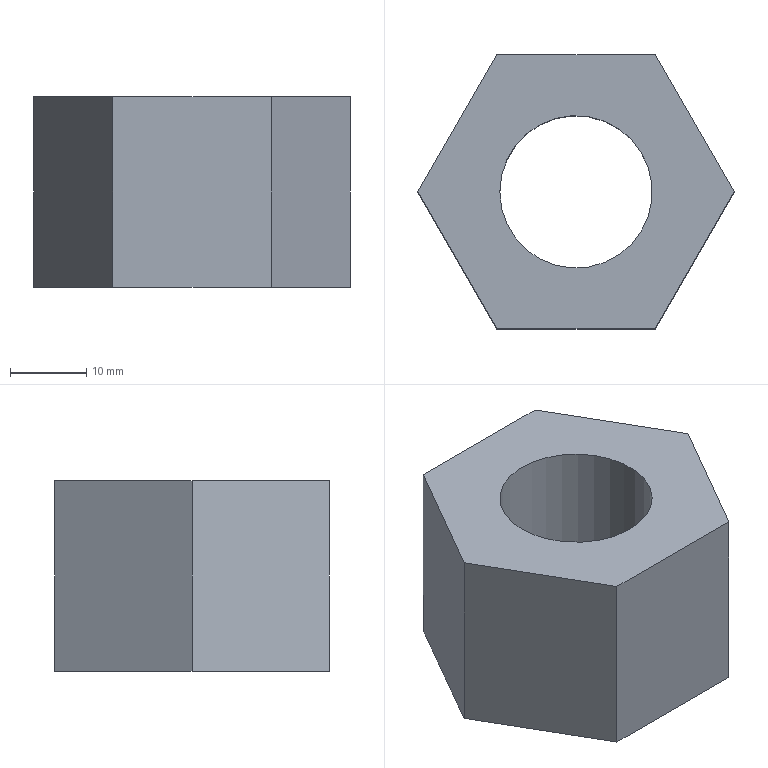Part | NX | features solid 2 | 1 solid | 9 faces | box 41.534 x 35.97 x 25 mm | volume 20158 mm3 | plane 8 | cylinder 1 | commonest cylinder face diameters 20 x1
STEP:
#1=CARTESIAN_POINT('',(-69.616,-457.985,-125.));
#2=VERTEX_POINT('',#1);
#3=CARTESIAN_POINT('',(-59.233,-440.,-125.));
#4=VERTEX_POINT('',#3);
#5=CARTESIAN_POINT('',(-73.081,-463.985,-125.));
#6=DIRECTION('',(0.5,0.866,0.));
#7=VECTOR('',#6,1000.);
#8=LINE('',#5,#7);
#9=EDGE_CURVE('',#2,#4,#8,.T.);
#10=ORIENTED_EDGE('',*,*,#9,.T.);
#11=CARTESIAN_POINT('',(-59.233,-440.,-100.));
#12=VERTEX_POINT('',#11);
#13=CARTESIAN_POINT('',(-59.233,-440.,-100.));
#14=DIRECTION('',(0.,0.,-1.));
#15=VECTOR('',#14,1000.);
#16=LINE('',#13,#15);
#17=EDGE_CURVE('',#12,#4,#16,.T.);
#18=ORIENTED_EDGE('',*,*,#17,.F.);
#19=CARTESIAN_POINT('',(-69.616,-457.985,-100.));
#20=VERTEX_POINT('',#19);
#21=CARTESIAN_POINT('',(-73.081,-463.985,-100.));
#22=DIRECTION('',(0.5,0.866,0.));
#23=VECTOR('',#22,1000.);
#24=LINE('',#21,#23);
#25=EDGE_CURVE('',#20,#12,#24,.T.);
#26=ORIENTED_EDGE('',*,*,#25,.F.);
#27=CARTESIAN_POINT('',(-69.616,-457.985,-100.));
#28=DIRECTION('',(0.,0.,-1.));
#29=VECTOR('',#28,1000.);
#30=LINE('',#27,#29);
#31=EDGE_CURVE('',#20,#2,#30,.T.);
#32=ORIENTED_EDGE('',*,*,#31,.T.);
#33=EDGE_LOOP('',(#10,#18,#26,#32));
#34=FACE_BOUND('',#33,.T.);
#35=CARTESIAN_POINT('',(-73.081,-463.985,-100.));
#36=DIRECTION('',(0.866,-0.5,0.));
#37=DIRECTION('',(0.5,0.866,0.));
#38=AXIS2_PLACEMENT_3D('',#35,#36,#37);
#39=PLANE('',#38);
#40=ADVANCED_FACE('',(#34),#39,.T.);
#41=CARTESIAN_POINT('',(-69.616,-422.015,-125.));
#42=VERTEX_POINT('',#41);
#43=CARTESIAN_POINT('',(-47.113,-460.992,-125.));
#44=DIRECTION('',(-0.5,0.866,0.));
#45=VECTOR('',#44,1000.);
#46=LINE('',#43,#45);
#47=EDGE_CURVE('',#4,#42,#46,.T.);
#48=ORIENTED_EDGE('',*,*,#47,.T.);
#49=CARTESIAN_POINT('',(-69.616,-422.015,-100.));
#50=VERTEX_POINT('',#49);
#51=CARTESIAN_POINT('',(-69.616,-422.015,-100.));
#52=DIRECTION('',(0.,0.,-1.));
#53=VECTOR('',#52,1000.);
#54=LINE('',#51,#53);
#55=EDGE_CURVE('',#50,#42,#54,.T.);
#56=ORIENTED_EDGE('',*,*,#55,.F.);
#57=CARTESIAN_POINT('',(-47.113,-460.992,-100.));
#58=DIRECTION('',(-0.5,0.866,0.));
#59=VECTOR('',#58,1000.);
#60=LINE('',#57,#59);
#61=EDGE_CURVE('',#12,#50,#60,.T.);
#62=ORIENTED_EDGE('',*,*,#61,.F.);
#63=ORIENTED_EDGE('',*,*,#17,.T.);
#64=EDGE_LOOP('',(#48,#56,#62,#63));
#65=FACE_BOUND('',#64,.T.);
#66=CARTESIAN_POINT('',(-55.769,-446.,-100.));
#67=DIRECTION('',(0.866,0.5,0.));
#68=DIRECTION('',(-0.5,0.866,0.));
#69=AXIS2_PLACEMENT_3D('',#66,#67,#68);
#70=PLANE('',#69);
#71=ADVANCED_FACE('',(#65),#70,.T.);
#72=CARTESIAN_POINT('',(-90.384,-422.015,-125.));
#73=VERTEX_POINT('',#72);
#74=CARTESIAN_POINT('',(-62.688,-422.015,-125.));
#75=DIRECTION('',(-1.,0.,0.));
#76=VECTOR('',#75,1000.);
#77=LINE('',#74,#76);
#78=EDGE_CURVE('',#42,#73,#77,.T.);
#79=ORIENTED_EDGE('',*,*,#78,.T.);
#80=CARTESIAN_POINT('',(-90.384,-422.015,-100.));
#81=VERTEX_POINT('',#80);
#82=CARTESIAN_POINT('',(-90.384,-422.015,-100.));
#83=DIRECTION('',(0.,0.,-1.));
#84=VECTOR('',#83,1000.);
#85=LINE('',#82,#84);
#86=EDGE_CURVE('',#81,#73,#85,.T.);
#87=ORIENTED_EDGE('',*,*,#86,.F.);
#88=CARTESIAN_POINT('',(-62.688,-422.015,-100.));
#89=DIRECTION('',(-1.,0.,0.));
#90=VECTOR('',#89,1000.);
#91=LINE('',#88,#90);
#92=EDGE_CURVE('',#50,#81,#91,.T.);
#93=ORIENTED_EDGE('',*,*,#92,.F.);
#94=ORIENTED_EDGE('',*,*,#55,.T.);
#95=EDGE_LOOP('',(#79,#87,#93,#94));
#96=FACE_BOUND('',#95,.T.);
#97=CARTESIAN_POINT('',(-62.688,-422.015,-100.));
#98=DIRECTION('',(0.,1.,0.));
#99=DIRECTION('',(-1.,0.,0.));
#100=AXIS2_PLACEMENT_3D('',#97,#98,#99);
#101=PLANE('',#100);
#102=ADVANCED_FACE('',(#96),#101,.T.);
#103=CARTESIAN_POINT('',(-100.767,-440.,-125.));
#104=VERTEX_POINT('',#103);
#105=CARTESIAN_POINT('',(-104.231,-446.,-125.));
#106=DIRECTION('',(-0.5,-0.866,0.));
#107=VECTOR('',#106,1000.);
#108=LINE('',#105,#107);
#109=EDGE_CURVE('',#73,#104,#108,.T.);
#110=ORIENTED_EDGE('',*,*,#109,.T.);
#111=CARTESIAN_POINT('',(-100.767,-440.,-100.));
#112=VERTEX_POINT('',#111);
#113=CARTESIAN_POINT('',(-100.767,-440.,-100.));
#114=DIRECTION('',(0.,0.,-1.));
#115=VECTOR('',#114,1000.);
#116=LINE('',#113,#115);
#117=EDGE_CURVE('',#112,#104,#116,.T.);
#118=ORIENTED_EDGE('',*,*,#117,.F.);
#119=CARTESIAN_POINT('',(-104.231,-446.,-100.));
#120=DIRECTION('',(-0.5,-0.866,0.));
#121=VECTOR('',#120,1000.);
#122=LINE('',#119,#121);
#123=EDGE_CURVE('',#81,#112,#122,.T.);
#124=ORIENTED_EDGE('',*,*,#123,.F.);
#125=ORIENTED_EDGE('',*,*,#86,.T.);
#126=EDGE_LOOP('',(#110,#118,#124,#125));
#127=FACE_BOUND('',#126,.T.);
#128=CARTESIAN_POINT('',(-86.919,-416.015,-100.));
#129=DIRECTION('',(-0.866,0.5,0.));
#130=DIRECTION('',(-0.5,-0.866,0.));
#131=AXIS2_PLACEMENT_3D('',#128,#129,#130);
#132=PLANE('',#131);
#133=ADVANCED_FACE('',(#127),#132,.T.);
#134=CARTESIAN_POINT('',(-90.384,-457.985,-125.));
#135=VERTEX_POINT('',#134);
#136=CARTESIAN_POINT('',(-78.264,-478.977,-125.));
#137=DIRECTION('',(0.5,-0.866,0.));
#138=VECTOR('',#137,1000.);
#139=LINE('',#136,#138);
#140=EDGE_CURVE('',#104,#135,#139,.T.);
#141=ORIENTED_EDGE('',*,*,#140,.T.);
#142=CARTESIAN_POINT('',(-90.384,-457.985,-100.));
#143=VERTEX_POINT('',#142);
#144=CARTESIAN_POINT('',(-90.384,-457.985,-100.));
#145=DIRECTION('',(0.,0.,-1.));
#146=VECTOR('',#145,1000.);
#147=LINE('',#144,#146);
#148=EDGE_CURVE('',#143,#135,#147,.T.);
#149=ORIENTED_EDGE('',*,*,#148,.F.);
#150=CARTESIAN_POINT('',(-78.264,-478.977,-100.));
#151=DIRECTION('',(0.5,-0.866,0.));
#152=VECTOR('',#151,1000.);
#153=LINE('',#150,#152);
#154=EDGE_CURVE('',#112,#143,#153,.T.);
#155=ORIENTED_EDGE('',*,*,#154,.F.);
#156=ORIENTED_EDGE('',*,*,#117,.T.);
#157=EDGE_LOOP('',(#141,#149,#155,#156));
#158=FACE_BOUND('',#157,.T.);
#159=CARTESIAN_POINT('',(-104.231,-434.,-100.));
#160=DIRECTION('',(-0.866,-0.5,0.));
#161=DIRECTION('',(0.5,-0.866,0.));
#162=AXIS2_PLACEMENT_3D('',#159,#160,#161);
#163=PLANE('',#162);
#164=ADVANCED_FACE('',(#158),#163,.T.);
#165=CARTESIAN_POINT('',(-90.,-440.,-100.));
#166=VERTEX_POINT('',#165);
#167=CARTESIAN_POINT('',(-80.,-440.,-100.));
#168=DIRECTION('',(0.,0.,1.));
#169=DIRECTION('',(-1.,0.,0.));
#170=AXIS2_PLACEMENT_3D('',#167,#168,#169);
#171=CIRCLE('',#170,10.);
#172=EDGE_CURVE('',#166,#166,#171,.T.);
#173=ORIENTED_EDGE('',*,*,#172,.T.);
#174=EDGE_LOOP('',(#173));
#175=FACE_BOUND('',#174,.T.);
#176=CARTESIAN_POINT('',(-90.,-440.,-125.));
#177=VERTEX_POINT('',#176);
#178=CARTESIAN_POINT('',(-80.,-440.,-125.));
#179=DIRECTION('',(0.,0.,1.));
#180=DIRECTION('',(-1.,0.,0.));
#181=AXIS2_PLACEMENT_3D('',#178,#179,#180);
#182=CIRCLE('',#181,10.);
#183=EDGE_CURVE('',#177,#177,#182,.T.);
#184=ORIENTED_EDGE('',*,*,#183,.F.);
#185=EDGE_LOOP('',(#184));
#186=FACE_BOUND('',#185,.T.);
#187=CARTESIAN_POINT('',(-80.,-440.,-100.));
#188=DIRECTION('',(0.,0.,-1.));
#189=DIRECTION('',(1.,0.,0.));
#190=AXIS2_PLACEMENT_3D('',#187,#188,#189);
#191=CYLINDRICAL_SURFACE('',#190,10.);
#192=ADVANCED_FACE('',(#175,#186),#191,.F.);
#193=CARTESIAN_POINT('',(-62.688,-457.985,-125.));
#194=DIRECTION('',(1.,0.,0.));
#195=VECTOR('',#194,1000.);
#196=LINE('',#193,#195);
#197=EDGE_CURVE('',#135,#2,#196,.T.);
#198=ORIENTED_EDGE('',*,*,#197,.T.);
#199=ORIENTED_EDGE('',*,*,#31,.F.);
#200=CARTESIAN_POINT('',(-62.688,-457.985,-100.));
#201=DIRECTION('',(1.,0.,0.));
#202=VECTOR('',#201,1000.);
#203=LINE('',#200,#202);
#204=EDGE_CURVE('',#143,#20,#203,.T.);
#205=ORIENTED_EDGE('',*,*,#204,.F.);
#206=ORIENTED_EDGE('',*,*,#148,.T.);
#207=EDGE_LOOP('',(#198,#199,#205,#206));
#208=FACE_BOUND('',#207,.T.);
#209=CARTESIAN_POINT('',(-97.312,-457.985,-100.));
#210=DIRECTION('',(0.,-1.,0.));
#211=DIRECTION('',(1.,0.,0.));
#212=AXIS2_PLACEMENT_3D('',#209,#210,#211);
#213=PLANE('',#212);
#214=ADVANCED_FACE('',(#208),#213,.T.);
#215=ORIENTED_EDGE('',*,*,#172,.F.);
#216=EDGE_LOOP('',(#215));
#217=FACE_BOUND('',#216,.T.);
#218=ORIENTED_EDGE('',*,*,#25,.T.);
#219=ORIENTED_EDGE('',*,*,#61,.T.);
#220=ORIENTED_EDGE('',*,*,#92,.T.);
#221=ORIENTED_EDGE('',*,*,#123,.T.);
#222=ORIENTED_EDGE('',*,*,#154,.T.);
#223=ORIENTED_EDGE('',*,*,#204,.T.);
#224=EDGE_LOOP('',(#218,#219,#220,#221,#222,#223));
#225=FACE_BOUND('',#224,.T.);
#226=CARTESIAN_POINT('',(-62.688,-469.985,-100.));
#227=DIRECTION('',(0.,0.,1.));
#228=DIRECTION('',(-1.,0.,0.));
#229=AXIS2_PLACEMENT_3D('',#226,#227,#228);
#230=PLANE('',#229);
#231=ADVANCED_FACE('',(#217,#225),#230,.T.);
#232=ORIENTED_EDGE('',*,*,#183,.T.);
#233=EDGE_LOOP('',(#232));
#234=FACE_BOUND('',#233,.T.);
#235=ORIENTED_EDGE('',*,*,#9,.F.);
#236=ORIENTED_EDGE('',*,*,#197,.F.);
#237=ORIENTED_EDGE('',*,*,#140,.F.);
#238=ORIENTED_EDGE('',*,*,#109,.F.);
#239=ORIENTED_EDGE('',*,*,#78,.F.);
#240=ORIENTED_EDGE('',*,*,#47,.F.);
#241=EDGE_LOOP('',(#235,#236,#237,#238,#239,#240));
#242=FACE_BOUND('',#241,.T.);
#243=CARTESIAN_POINT('',(-62.688,-469.985,-125.));
#244=DIRECTION('',(0.,0.,1.));
#245=DIRECTION('',(-1.,0.,0.));
#246=AXIS2_PLACEMENT_3D('',#243,#244,#245);
#247=PLANE('',#246);
#248=ADVANCED_FACE('',(#234,#242),#247,.F.);
#249=CLOSED_SHELL('',(#40,#71,#102,#133,#164,#192,#214,#231,#248));
#250=MANIFOLD_SOLID_BREP('',#249);
#251=(LENGTH_UNIT()NAMED_UNIT(*)SI_UNIT(.MILLI.,.METRE.));
#252=UNCERTAINTY_MEASURE_WITH_UNIT(LENGTH_MEASURE(0.00001),#251,'','');
#253=(NAMED_UNIT(*)PLANE_ANGLE_UNIT()SI_UNIT($,.RADIAN.));
#254=(NAMED_UNIT(*)SI_UNIT($,.STERADIAN.)SOLID_ANGLE_UNIT());
#255=(GEOMETRIC_REPRESENTATION_CONTEXT(3)GLOBAL_UNCERTAINTY_ASSIGNED_CONTEXT((#252))GLOBAL_UNIT_ASSIGNED_CONTEXT((#251,#253,#254))REPRESENTATION_CONTEXT('',''));
#256=ADVANCED_BREP_SHAPE_REPRESENTATION('',(#250),#255);